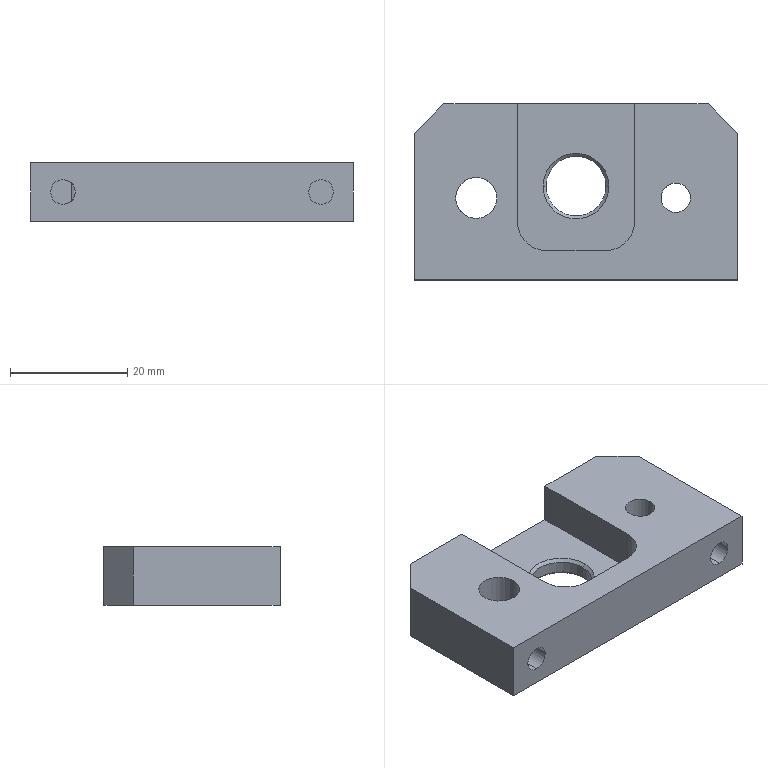Part | STEP file | PN_0072 Mount electronic clip s longitudinal manipulator cylinder seat | 1 solid | 30 faces | box 55 x 30 x 10 mm | volume 11604 mm3 | plane 14 | cylinder 12 | cone 4 | commonest cylinder face diameters 4.2 x4 5 x2 7 x2 10 x2 10.2 x2